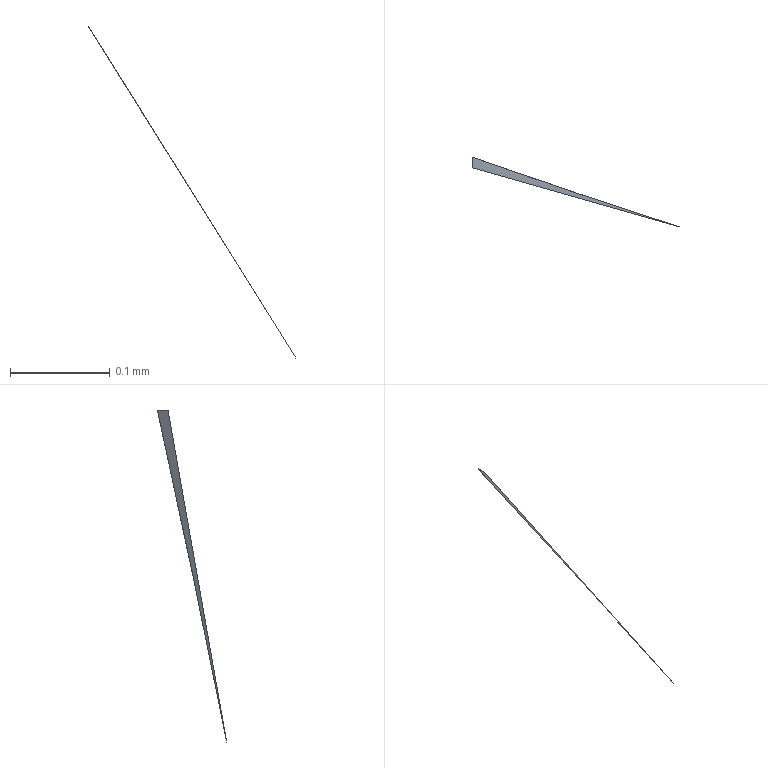Part | Creo | 1 solid | 4 faces | box 0.2078 x 0.06932 x 0.3326 mm | volume 0.000000109 mm3 | plane 3 | spline 1